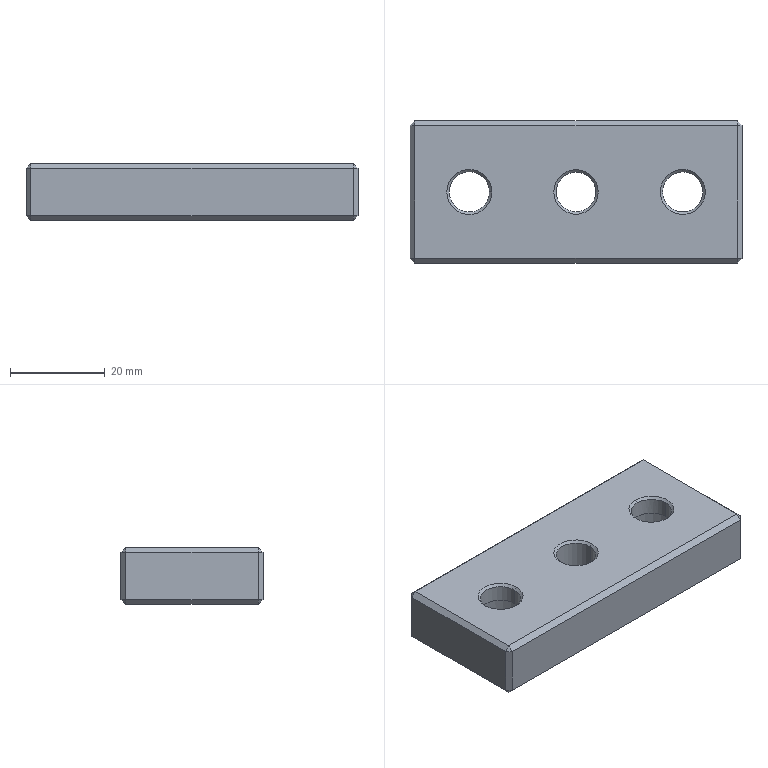Part | STEP file | Adjusting plate | 1 solid | 50 faces | box 70 x 30 x 12 mm | volume 21378 mm3 | plane 28 | cone 12 | cylinder 10 | commonest cylinder face diameters 8.5 x4 14 x4 8.376 x2